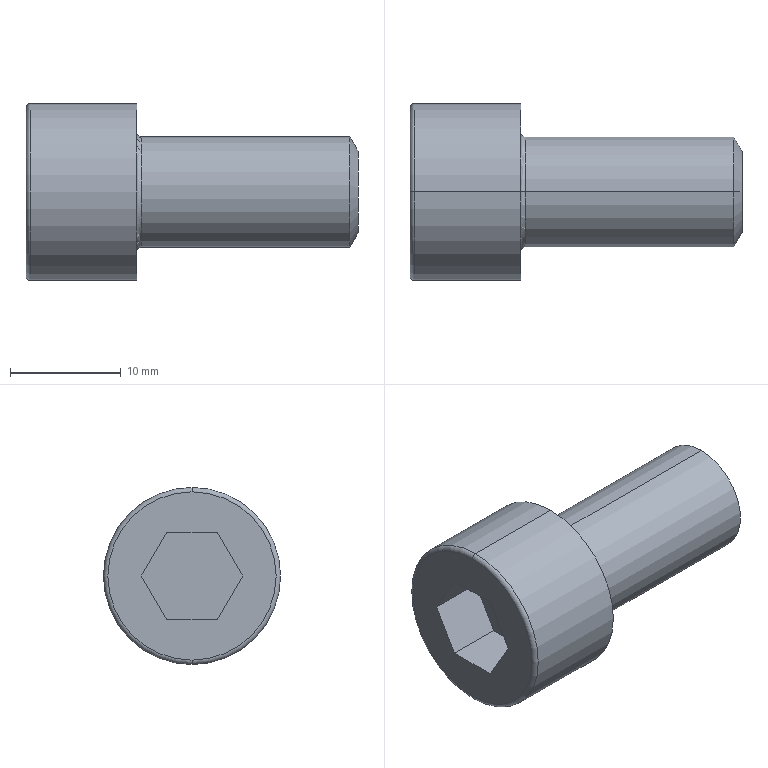Part | SolidWorks | features BlendCut 1, Cut 1, Fillet 1, LPattern 1, RevCut 1, Revolution 1 | 1 solid | 20 faces | box 30 x 16 x 16 mm | volume 3295 mm3 | plane 10 | torus 4 | cylinder 4 | cone 2 | commonest cylinder face diameters 10 x2 16 x2
STEP:
#1=CARTESIAN_POINT('',(30.,0.,3.701));
#2=VERTEX_POINT('',#1);
#3=CARTESIAN_POINT('',(30.,0.,-3.701));
#4=VERTEX_POINT('',#3);
#5=CARTESIAN_POINT('',(30.,0.,0.));
#6=DIRECTION('',(-1.,0.,0.));
#7=DIRECTION('',(0.,0.,1.));
#8=AXIS2_PLACEMENT_3D('',#5,#6,#7);
#9=CIRCLE('',#8,3.701);
#10=EDGE_CURVE('',#2,#4,#9,.T.);
#11=ORIENTED_EDGE('',*,*,#10,.T.);
#12=CARTESIAN_POINT('',(29.25,0.,-5.));
#13=VERTEX_POINT('',#12);
#14=CARTESIAN_POINT('',(29.25,0.,-5.));
#15=DIRECTION('',(-0.5,0.,-0.866));
#16=VECTOR('',#15,1000.);
#17=LINE('',#14,#16);
#18=EDGE_CURVE('',#4,#13,#17,.T.);
#19=ORIENTED_EDGE('',*,*,#18,.T.);
#20=CARTESIAN_POINT('',(29.25,0.,5.));
#21=VERTEX_POINT('',#20);
#22=CARTESIAN_POINT('',(29.25,0.,0.));
#23=DIRECTION('',(-1.,0.,0.));
#24=DIRECTION('',(0.,0.,1.));
#25=AXIS2_PLACEMENT_3D('',#22,#23,#24);
#26=CIRCLE('',#25,5.);
#27=EDGE_CURVE('',#21,#13,#26,.T.);
#28=ORIENTED_EDGE('',*,*,#27,.F.);
#29=CARTESIAN_POINT('',(29.25,0.,5.));
#30=DIRECTION('',(-0.5,0.,0.866));
#31=VECTOR('',#30,1000.);
#32=LINE('',#29,#31);
#33=EDGE_CURVE('',#2,#21,#32,.T.);
#34=ORIENTED_EDGE('',*,*,#33,.F.);
#35=EDGE_LOOP('',(#11,#19,#28,#34));
#36=FACE_OUTER_BOUND('',#35,.T.);
#37=CARTESIAN_POINT('',(29.25,0.,0.));
#38=DIRECTION('',(-1.,0.,0.));
#39=DIRECTION('',(0.,0.,1.));
#40=AXIS2_PLACEMENT_3D('',#37,#38,#39);
#41=CONICAL_SURFACE('',#40,5.,1.047);
#42=ADVANCED_FACE('',(#36),#41,.T.);
#43=CARTESIAN_POINT('',(0.4,0.,-8.));
#44=VERTEX_POINT('',#43);
#45=CARTESIAN_POINT('',(0.4,0.,8.));
#46=VERTEX_POINT('',#45);
#47=CARTESIAN_POINT('',(0.4,0.,0.));
#48=DIRECTION('',(1.,0.,0.));
#49=DIRECTION('',(0.,0.,1.));
#50=AXIS2_PLACEMENT_3D('',#47,#48,#49);
#51=CIRCLE('',#50,8.);
#52=EDGE_CURVE('',#44,#46,#51,.T.);
#53=ORIENTED_EDGE('',*,*,#52,.F.);
#54=CARTESIAN_POINT('',(0.,0.,-7.6));
#55=VERTEX_POINT('',#54);
#56=CARTESIAN_POINT('',(0.4,0.,-7.6));
#57=DIRECTION('',(0.,1.,0.));
#58=DIRECTION('',(0.,0.,1.));
#59=AXIS2_PLACEMENT_3D('',#56,#57,#58);
#60=CIRCLE('',#59,0.4);
#61=EDGE_CURVE('',#44,#55,#60,.T.);
#62=ORIENTED_EDGE('',*,*,#61,.T.);
#63=CARTESIAN_POINT('',(0.,0.,7.6));
#64=VERTEX_POINT('',#63);
#65=CARTESIAN_POINT('',(0.,0.,0.));
#66=DIRECTION('',(-1.,0.,0.));
#67=DIRECTION('',(0.,0.,1.));
#68=AXIS2_PLACEMENT_3D('',#65,#66,#67);
#69=CIRCLE('',#68,7.6);
#70=EDGE_CURVE('',#64,#55,#69,.T.);
#71=ORIENTED_EDGE('',*,*,#70,.F.);
#72=CARTESIAN_POINT('',(0.4,0.,7.6));
#73=DIRECTION('',(0.,-1.,0.));
#74=DIRECTION('',(0.,0.,-1.));
#75=AXIS2_PLACEMENT_3D('',#72,#73,#74);
#76=CIRCLE('',#75,0.4);
#77=EDGE_CURVE('',#46,#64,#76,.T.);
#78=ORIENTED_EDGE('',*,*,#77,.F.);
#79=EDGE_LOOP('',(#53,#62,#71,#78));
#80=FACE_OUTER_BOUND('',#79,.T.);
#81=CARTESIAN_POINT('',(0.4,0.,0.));
#82=DIRECTION('',(-1.,0.,0.));
#83=DIRECTION('',(0.,0.,1.));
#84=AXIS2_PLACEMENT_3D('',#81,#82,#83);
#85=TOROIDAL_SURFACE('',#84,7.6,0.4);
#86=ADVANCED_FACE('',(#80),#85,.T.);
#87=CARTESIAN_POINT('',(10.4,0.,5.));
#88=VERTEX_POINT('',#87);
#89=CARTESIAN_POINT('',(10.4,0.,-5.));
#90=VERTEX_POINT('',#89);
#91=CARTESIAN_POINT('',(10.4,0.,0.));
#92=DIRECTION('',(1.,0.,0.));
#93=DIRECTION('',(0.,0.,-1.));
#94=AXIS2_PLACEMENT_3D('',#91,#92,#93);
#95=CIRCLE('',#94,5.);
#96=EDGE_CURVE('',#88,#90,#95,.T.);
#97=ORIENTED_EDGE('',*,*,#96,.F.);
#98=CARTESIAN_POINT('',(10.,0.,5.4));
#99=VERTEX_POINT('',#98);
#100=CARTESIAN_POINT('',(10.4,0.,5.4));
#101=DIRECTION('',(0.,1.,0.));
#102=DIRECTION('',(0.,0.,1.));
#103=AXIS2_PLACEMENT_3D('',#100,#101,#102);
#104=CIRCLE('',#103,0.4);
#105=EDGE_CURVE('',#88,#99,#104,.T.);
#106=ORIENTED_EDGE('',*,*,#105,.T.);
#107=CARTESIAN_POINT('',(10.,0.,-5.4));
#108=VERTEX_POINT('',#107);
#109=CARTESIAN_POINT('',(10.,0.,0.));
#110=DIRECTION('',(1.,0.,0.));
#111=DIRECTION('',(0.,0.,-1.));
#112=AXIS2_PLACEMENT_3D('',#109,#110,#111);
#113=CIRCLE('',#112,5.4);
#114=EDGE_CURVE('',#99,#108,#113,.T.);
#115=ORIENTED_EDGE('',*,*,#114,.T.);
#116=CARTESIAN_POINT('',(10.4,0.,-5.4));
#117=DIRECTION('',(0.,-1.,0.));
#118=DIRECTION('',(0.,0.,-1.));
#119=AXIS2_PLACEMENT_3D('',#116,#117,#118);
#120=CIRCLE('',#119,0.4);
#121=EDGE_CURVE('',#90,#108,#120,.T.);
#122=ORIENTED_EDGE('',*,*,#121,.F.);
#123=EDGE_LOOP('',(#97,#106,#115,#122));
#124=FACE_OUTER_BOUND('',#123,.T.);
#125=CARTESIAN_POINT('',(10.4,0.,0.));
#126=DIRECTION('',(1.,0.,0.));
#127=DIRECTION('',(0.,0.,-1.));
#128=AXIS2_PLACEMENT_3D('',#125,#126,#127);
#129=TOROIDAL_SURFACE('',#128,5.4,0.4);
#130=ADVANCED_FACE('',(#124),#129,.F.);
#131=ORIENTED_EDGE('',*,*,#52,.T.);
#132=CARTESIAN_POINT('',(10.,0.,8.));
#133=VERTEX_POINT('',#132);
#134=CARTESIAN_POINT('',(0.,0.,8.));
#135=DIRECTION('',(1.,0.,0.));
#136=VECTOR('',#135,1000.);
#137=LINE('',#134,#136);
#138=EDGE_CURVE('',#46,#133,#137,.T.);
#139=ORIENTED_EDGE('',*,*,#138,.T.);
#140=CARTESIAN_POINT('',(10.,0.,-8.));
#141=VERTEX_POINT('',#140);
#142=CARTESIAN_POINT('',(10.,0.,0.));
#143=DIRECTION('',(1.,0.,0.));
#144=DIRECTION('',(0.,0.,-1.));
#145=AXIS2_PLACEMENT_3D('',#142,#143,#144);
#146=CIRCLE('',#145,8.);
#147=EDGE_CURVE('',#141,#133,#146,.T.);
#148=ORIENTED_EDGE('',*,*,#147,.F.);
#149=CARTESIAN_POINT('',(0.,0.,-8.));
#150=DIRECTION('',(1.,0.,0.));
#151=VECTOR('',#150,1000.);
#152=LINE('',#149,#151);
#153=EDGE_CURVE('',#44,#141,#152,.T.);
#154=ORIENTED_EDGE('',*,*,#153,.F.);
#155=EDGE_LOOP('',(#131,#139,#148,#154));
#156=FACE_OUTER_BOUND('',#155,.T.);
#157=CARTESIAN_POINT('',(0.,0.,0.));
#158=DIRECTION('',(1.,0.,0.));
#159=DIRECTION('',(0.,0.,-1.));
#160=AXIS2_PLACEMENT_3D('',#157,#158,#159);
#161=CYLINDRICAL_SURFACE('',#160,8.);
#162=ADVANCED_FACE('',(#156),#161,.T.);
#163=CARTESIAN_POINT('',(10.4,0.,0.));
#164=DIRECTION('',(1.,0.,0.));
#165=DIRECTION('',(0.,0.,-1.));
#166=AXIS2_PLACEMENT_3D('',#163,#164,#165);
#167=CIRCLE('',#166,5.);
#168=EDGE_CURVE('',#90,#88,#167,.T.);
#169=ORIENTED_EDGE('',*,*,#168,.T.);
#170=CARTESIAN_POINT('',(0.,0.,5.));
#171=DIRECTION('',(1.,0.,0.));
#172=VECTOR('',#171,1000.);
#173=LINE('',#170,#172);
#174=EDGE_CURVE('',#88,#21,#173,.T.);
#175=ORIENTED_EDGE('',*,*,#174,.T.);
#176=ORIENTED_EDGE('',*,*,#27,.T.);
#177=CARTESIAN_POINT('',(0.,0.,-5.));
#178=DIRECTION('',(1.,0.,0.));
#179=VECTOR('',#178,1000.);
#180=LINE('',#177,#179);
#181=EDGE_CURVE('',#90,#13,#180,.T.);
#182=ORIENTED_EDGE('',*,*,#181,.F.);
#183=EDGE_LOOP('',(#169,#175,#176,#182));
#184=FACE_OUTER_BOUND('',#183,.T.);
#185=CARTESIAN_POINT('',(0.,0.,0.));
#186=DIRECTION('',(1.,0.,0.));
#187=DIRECTION('',(0.,0.,-1.));
#188=AXIS2_PLACEMENT_3D('',#185,#186,#187);
#189=CYLINDRICAL_SURFACE('',#188,5.);
#190=ADVANCED_FACE('',(#184),#189,.T.);
#191=ORIENTED_EDGE('',*,*,#174,.F.);
#192=ORIENTED_EDGE('',*,*,#96,.T.);
#193=ORIENTED_EDGE('',*,*,#181,.T.);
#194=CARTESIAN_POINT('',(29.25,0.,0.));
#195=DIRECTION('',(-1.,0.,0.));
#196=DIRECTION('',(0.,0.,1.));
#197=AXIS2_PLACEMENT_3D('',#194,#195,#196);
#198=CIRCLE('',#197,5.);
#199=EDGE_CURVE('',#13,#21,#198,.T.);
#200=ORIENTED_EDGE('',*,*,#199,.T.);
#201=EDGE_LOOP('',(#191,#192,#193,#200));
#202=FACE_OUTER_BOUND('',#201,.T.);
#203=CARTESIAN_POINT('',(0.,0.,0.));
#204=DIRECTION('',(1.,0.,0.));
#205=DIRECTION('',(0.,0.,-1.));
#206=AXIS2_PLACEMENT_3D('',#203,#204,#205);
#207=CYLINDRICAL_SURFACE('',#206,5.);
#208=ADVANCED_FACE('',(#202),#207,.T.);
#209=ORIENTED_EDGE('',*,*,#70,.T.);
#210=CARTESIAN_POINT('',(0.,0.,0.));
#211=DIRECTION('',(-1.,0.,0.));
#212=DIRECTION('',(0.,0.,1.));
#213=AXIS2_PLACEMENT_3D('',#210,#211,#212);
#214=CIRCLE('',#213,7.6);
#215=EDGE_CURVE('',#55,#64,#214,.T.);
#216=ORIENTED_EDGE('',*,*,#215,.T.);
#217=EDGE_LOOP('',(#209,#216));
#218=FACE_OUTER_BOUND('',#217,.T.);
#219=CARTESIAN_POINT('',(0.,-4.575,0.));
#220=VERTEX_POINT('',#219);
#221=CARTESIAN_POINT('',(0.,-2.288,3.962));
#222=VERTEX_POINT('',#221);
#223=CARTESIAN_POINT('',(0.,-4.575,0.));
#224=DIRECTION('',(0.,0.5,0.866));
#225=VECTOR('',#224,1000.);
#226=LINE('',#223,#225);
#227=EDGE_CURVE('',#220,#222,#226,.T.);
#228=ORIENTED_EDGE('',*,*,#227,.F.);
#229=CARTESIAN_POINT('',(0.,-2.288,-3.962));
#230=VERTEX_POINT('',#229);
#231=CARTESIAN_POINT('',(0.,-2.288,-3.962));
#232=DIRECTION('',(0.,-0.5,0.866));
#233=VECTOR('',#232,1000.);
#234=LINE('',#231,#233);
#235=EDGE_CURVE('',#230,#220,#234,.T.);
#236=ORIENTED_EDGE('',*,*,#235,.F.);
#237=CARTESIAN_POINT('',(0.,2.288,-3.962));
#238=VERTEX_POINT('',#237);
#239=CARTESIAN_POINT('',(0.,2.288,-3.962));
#240=DIRECTION('',(0.,-1.,0.));
#241=VECTOR('',#240,1000.);
#242=LINE('',#239,#241);
#243=EDGE_CURVE('',#238,#230,#242,.T.);
#244=ORIENTED_EDGE('',*,*,#243,.F.);
#245=CARTESIAN_POINT('',(0.,4.575,0.));
#246=VERTEX_POINT('',#245);
#247=CARTESIAN_POINT('',(0.,4.575,0.));
#248=DIRECTION('',(0.,-0.5,-0.866));
#249=VECTOR('',#248,1000.);
#250=LINE('',#247,#249);
#251=EDGE_CURVE('',#246,#238,#250,.T.);
#252=ORIENTED_EDGE('',*,*,#251,.F.);
#253=CARTESIAN_POINT('',(0.,2.288,3.962));
#254=VERTEX_POINT('',#253);
#255=CARTESIAN_POINT('',(0.,2.288,3.962));
#256=DIRECTION('',(0.,0.5,-0.866));
#257=VECTOR('',#256,1000.);
#258=LINE('',#255,#257);
#259=EDGE_CURVE('',#254,#246,#258,.T.);
#260=ORIENTED_EDGE('',*,*,#259,.F.);
#261=CARTESIAN_POINT('',(0.,-2.288,3.962));
#262=DIRECTION('',(0.,1.,0.));
#263=VECTOR('',#262,1000.);
#264=LINE('',#261,#263);
#265=EDGE_CURVE('',#222,#254,#264,.T.);
#266=ORIENTED_EDGE('',*,*,#265,.F.);
#267=EDGE_LOOP('',(#228,#236,#244,#252,#260,#266));
#268=FACE_BOUND('',#267,.T.);
#269=CARTESIAN_POINT('',(0.,0.,0.));
#270=DIRECTION('',(-1.,0.,0.));
#271=DIRECTION('',(0.,0.,1.));
#272=AXIS2_PLACEMENT_3D('',#269,#270,#271);
#273=PLANE('',#272);
#274=ADVANCED_FACE('',(#218,#268),#273,.T.);
#275=ORIENTED_EDGE('',*,*,#138,.F.);
#276=CARTESIAN_POINT('',(0.4,0.,0.));
#277=DIRECTION('',(1.,0.,0.));
#278=DIRECTION('',(0.,0.,1.));
#279=AXIS2_PLACEMENT_3D('',#276,#277,#278);
#280=CIRCLE('',#279,8.);
#281=EDGE_CURVE('',#46,#44,#280,.T.);
#282=ORIENTED_EDGE('',*,*,#281,.T.);
#283=ORIENTED_EDGE('',*,*,#153,.T.);
#284=CARTESIAN_POINT('',(10.,0.,0.));
#285=DIRECTION('',(1.,0.,0.));
#286=DIRECTION('',(0.,0.,-1.));
#287=AXIS2_PLACEMENT_3D('',#284,#285,#286);
#288=CIRCLE('',#287,8.);
#289=EDGE_CURVE('',#133,#141,#288,.T.);
#290=ORIENTED_EDGE('',*,*,#289,.F.);
#291=EDGE_LOOP('',(#275,#282,#283,#290));
#292=FACE_OUTER_BOUND('',#291,.T.);
#293=CARTESIAN_POINT('',(0.,0.,0.));
#294=DIRECTION('',(1.,0.,0.));
#295=DIRECTION('',(0.,0.,-1.));
#296=AXIS2_PLACEMENT_3D('',#293,#294,#295);
#297=CYLINDRICAL_SURFACE('',#296,8.);
#298=ADVANCED_FACE('',(#292),#297,.T.);
#299=ORIENTED_EDGE('',*,*,#147,.T.);
#300=ORIENTED_EDGE('',*,*,#289,.T.);
#301=EDGE_LOOP('',(#299,#300));
#302=FACE_OUTER_BOUND('',#301,.T.);
#303=CARTESIAN_POINT('',(10.,0.,0.));
#304=DIRECTION('',(1.,0.,0.));
#305=DIRECTION('',(0.,0.,-1.));
#306=AXIS2_PLACEMENT_3D('',#303,#304,#305);
#307=CIRCLE('',#306,5.4);
#308=EDGE_CURVE('',#108,#99,#307,.T.);
#309=ORIENTED_EDGE('',*,*,#308,.F.);
#310=ORIENTED_EDGE('',*,*,#114,.F.);
#311=EDGE_LOOP('',(#309,#310));
#312=FACE_BOUND('',#311,.T.);
#313=CARTESIAN_POINT('',(10.,8.,0.));
#314=DIRECTION('',(1.,0.,0.));
#315=DIRECTION('',(0.,0.,-1.));
#316=AXIS2_PLACEMENT_3D('',#313,#314,#315);
#317=PLANE('',#316);
#318=ADVANCED_FACE('',(#302,#312),#317,.T.);
#319=ORIENTED_EDGE('',*,*,#105,.F.);
#320=ORIENTED_EDGE('',*,*,#168,.F.);
#321=ORIENTED_EDGE('',*,*,#121,.T.);
#322=ORIENTED_EDGE('',*,*,#308,.T.);
#323=EDGE_LOOP('',(#319,#320,#321,#322));
#324=FACE_OUTER_BOUND('',#323,.T.);
#325=CARTESIAN_POINT('',(10.4,0.,0.));
#326=DIRECTION('',(1.,0.,0.));
#327=DIRECTION('',(0.,0.,-1.));
#328=AXIS2_PLACEMENT_3D('',#325,#326,#327);
#329=TOROIDAL_SURFACE('',#328,5.4,0.4);
#330=ADVANCED_FACE('',(#324),#329,.F.);
#331=ORIENTED_EDGE('',*,*,#227,.T.);
#332=CARTESIAN_POINT('',(5.,-2.288,3.962));
#333=VERTEX_POINT('',#332);
#334=CARTESIAN_POINT('',(5.,-2.288,3.962));
#335=DIRECTION('',(-1.,0.,0.));
#336=VECTOR('',#335,1000.);
#337=LINE('',#334,#336);
#338=EDGE_CURVE('',#333,#222,#337,.T.);
#339=ORIENTED_EDGE('',*,*,#338,.F.);
#340=CARTESIAN_POINT('',(5.,-4.575,0.));
#341=VERTEX_POINT('',#340);
#342=CARTESIAN_POINT('',(5.,-4.575,0.));
#343=DIRECTION('',(0.,0.5,0.866));
#344=VECTOR('',#343,1000.);
#345=LINE('',#342,#344);
#346=EDGE_CURVE('',#341,#333,#345,.T.);
#347=ORIENTED_EDGE('',*,*,#346,.F.);
#348=CARTESIAN_POINT('',(5.,-4.575,0.));
#349=DIRECTION('',(-1.,0.,0.));
#350=VECTOR('',#349,1000.);
#351=LINE('',#348,#350);
#352=EDGE_CURVE('',#341,#220,#351,.T.);
#353=ORIENTED_EDGE('',*,*,#352,.T.);
#354=EDGE_LOOP('',(#331,#339,#347,#353));
#355=FACE_OUTER_BOUND('',#354,.T.);
#356=CARTESIAN_POINT('',(5.,-4.575,0.));
#357=DIRECTION('',(0.,-0.866,0.5));
#358=DIRECTION('',(0.,-0.5,-0.866));
#359=AXIS2_PLACEMENT_3D('',#356,#357,#358);
#360=PLANE('',#359);
#361=ADVANCED_FACE('',(#355),#360,.F.);
#362=ORIENTED_EDGE('',*,*,#235,.T.);
#363=ORIENTED_EDGE('',*,*,#352,.F.);
#364=CARTESIAN_POINT('',(5.,-2.288,-3.962));
#365=VERTEX_POINT('',#364);
#366=CARTESIAN_POINT('',(5.,-2.288,-3.962));
#367=DIRECTION('',(0.,-0.5,0.866));
#368=VECTOR('',#367,1000.);
#369=LINE('',#366,#368);
#370=EDGE_CURVE('',#365,#341,#369,.T.);
#371=ORIENTED_EDGE('',*,*,#370,.F.);
#372=CARTESIAN_POINT('',(5.,-2.288,-3.962));
#373=DIRECTION('',(-1.,0.,0.));
#374=VECTOR('',#373,1000.);
#375=LINE('',#372,#374);
#376=EDGE_CURVE('',#365,#230,#375,.T.);
#377=ORIENTED_EDGE('',*,*,#376,.T.);
#378=EDGE_LOOP('',(#362,#363,#371,#377));
#379=FACE_OUTER_BOUND('',#378,.T.);
#380=CARTESIAN_POINT('',(5.,-2.288,-3.962));
#381=DIRECTION('',(0.,-0.866,-0.5));
#382=DIRECTION('',(0.,0.5,-0.866));
#383=AXIS2_PLACEMENT_3D('',#380,#381,#382);
#384=PLANE('',#383);
#385=ADVANCED_FACE('',(#379),#384,.F.);
#386=ORIENTED_EDGE('',*,*,#243,.T.);
#387=ORIENTED_EDGE('',*,*,#376,.F.);
#388=CARTESIAN_POINT('',(5.,2.288,-3.962));
#389=VERTEX_POINT('',#388);
#390=CARTESIAN_POINT('',(5.,2.288,-3.962));
#391=DIRECTION('',(0.,-1.,0.));
#392=VECTOR('',#391,1000.);
#393=LINE('',#390,#392);
#394=EDGE_CURVE('',#389,#365,#393,.T.);
#395=ORIENTED_EDGE('',*,*,#394,.F.);
#396=CARTESIAN_POINT('',(5.,2.288,-3.962));
#397=DIRECTION('',(-1.,0.,0.));
#398=VECTOR('',#397,1000.);
#399=LINE('',#396,#398);
#400=EDGE_CURVE('',#389,#238,#399,.T.);
#401=ORIENTED_EDGE('',*,*,#400,.T.);
#402=EDGE_LOOP('',(#386,#387,#395,#401));
#403=FACE_OUTER_BOUND('',#402,.T.);
#404=CARTESIAN_POINT('',(5.,2.288,-3.962));
#405=DIRECTION('',(0.,0.,-1.));
#406=DIRECTION('',(0.,1.,0.));
#407=AXIS2_PLACEMENT_3D('',#404,#405,#406);
#408=PLANE('',#407);
#409=ADVANCED_FACE('',(#403),#408,.F.);
#410=ORIENTED_EDGE('',*,*,#251,.T.);
#411=ORIENTED_EDGE('',*,*,#400,.F.);
#412=CARTESIAN_POINT('',(5.,4.575,0.));
#413=VERTEX_POINT('',#412);
#414=CARTESIAN_POINT('',(5.,4.575,0.));
#415=DIRECTION('',(0.,-0.5,-0.866));
#416=VECTOR('',#415,1000.);
#417=LINE('',#414,#416);
#418=EDGE_CURVE('',#413,#389,#417,.T.);
#419=ORIENTED_EDGE('',*,*,#418,.F.);
#420=CARTESIAN_POINT('',(5.,4.575,0.));
#421=DIRECTION('',(-1.,0.,0.));
#422=VECTOR('',#421,1000.);
#423=LINE('',#420,#422);
#424=EDGE_CURVE('',#413,#246,#423,.T.);
#425=ORIENTED_EDGE('',*,*,#424,.T.);
#426=EDGE_LOOP('',(#410,#411,#419,#425));
#427=FACE_OUTER_BOUND('',#426,.T.);
#428=CARTESIAN_POINT('',(5.,4.575,0.));
#429=DIRECTION('',(0.,0.866,-0.5));
#430=DIRECTION('',(0.,0.5,0.866));
#431=AXIS2_PLACEMENT_3D('',#428,#429,#430);
#432=PLANE('',#431);
#433=ADVANCED_FACE('',(#427),#432,.F.);
#434=ORIENTED_EDGE('',*,*,#259,.T.);
#435=ORIENTED_EDGE('',*,*,#424,.F.);
#436=CARTESIAN_POINT('',(5.,2.288,3.962));
#437=VERTEX_POINT('',#436);
#438=CARTESIAN_POINT('',(5.,2.288,3.962));
#439=DIRECTION('',(0.,0.5,-0.866));
#440=VECTOR('',#439,1000.);
#441=LINE('',#438,#440);
#442=EDGE_CURVE('',#437,#413,#441,.T.);
#443=ORIENTED_EDGE('',*,*,#442,.F.);
#444=CARTESIAN_POINT('',(5.,2.288,3.962));
#445=DIRECTION('',(-1.,0.,0.));
#446=VECTOR('',#445,1000.);
#447=LINE('',#444,#446);
#448=EDGE_CURVE('',#437,#254,#447,.T.);
#449=ORIENTED_EDGE('',*,*,#448,.T.);
#450=EDGE_LOOP('',(#434,#435,#443,#449));
#451=FACE_OUTER_BOUND('',#450,.T.);
#452=CARTESIAN_POINT('',(5.,2.288,3.962));
#453=DIRECTION('',(0.,0.866,0.5));
#454=DIRECTION('',(0.,-0.5,0.866));
#455=AXIS2_PLACEMENT_3D('',#452,#453,#454);
#456=PLANE('',#455);
#457=ADVANCED_FACE('',(#451),#456,.F.);
#458=ORIENTED_EDGE('',*,*,#265,.T.);
#459=ORIENTED_EDGE('',*,*,#448,.F.);
#460=CARTESIAN_POINT('',(5.,-2.288,3.962));
#461=DIRECTION('',(0.,1.,0.));
#462=VECTOR('',#461,1000.);
#463=LINE('',#460,#462);
#464=EDGE_CURVE('',#333,#437,#463,.T.);
#465=ORIENTED_EDGE('',*,*,#464,.F.);
#466=ORIENTED_EDGE('',*,*,#338,.T.);
#467=EDGE_LOOP('',(#458,#459,#465,#466));
#468=FACE_OUTER_BOUND('',#467,.T.);
#469=CARTESIAN_POINT('',(5.,-2.288,3.962));
#470=DIRECTION('',(0.,0.,1.));
#471=DIRECTION('',(0.,-1.,0.));
#472=AXIS2_PLACEMENT_3D('',#469,#470,#471);
#473=PLANE('',#472);
#474=ADVANCED_FACE('',(#468),#473,.F.);
#475=ORIENTED_EDGE('',*,*,#346,.T.);
#476=ORIENTED_EDGE('',*,*,#464,.T.);
#477=ORIENTED_EDGE('',*,*,#442,.T.);
#478=ORIENTED_EDGE('',*,*,#418,.T.);
#479=ORIENTED_EDGE('',*,*,#394,.T.);
#480=ORIENTED_EDGE('',*,*,#370,.T.);
#481=EDGE_LOOP('',(#475,#476,#477,#478,#479,#480));
#482=FACE_OUTER_BOUND('',#481,.T.);
#483=CARTESIAN_POINT('',(5.,-2.288,3.962));
#484=DIRECTION('',(-1.,0.,0.));
#485=DIRECTION('',(0.,0.,1.));
#486=AXIS2_PLACEMENT_3D('',#483,#484,#485);
#487=PLANE('',#486);
#488=ADVANCED_FACE('',(#482),#487,.T.);
#489=ORIENTED_EDGE('',*,*,#61,.F.);
#490=ORIENTED_EDGE('',*,*,#281,.F.);
#491=ORIENTED_EDGE('',*,*,#77,.T.);
#492=ORIENTED_EDGE('',*,*,#215,.F.);
#493=EDGE_LOOP('',(#489,#490,#491,#492));
#494=FACE_OUTER_BOUND('',#493,.T.);
#495=CARTESIAN_POINT('',(0.4,0.,0.));
#496=DIRECTION('',(-1.,0.,0.));
#497=DIRECTION('',(0.,0.,1.));
#498=AXIS2_PLACEMENT_3D('',#495,#496,#497);
#499=TOROIDAL_SURFACE('',#498,7.6,0.4);
#500=ADVANCED_FACE('',(#494),#499,.T.);
#501=ORIENTED_EDGE('',*,*,#18,.F.);
#502=CARTESIAN_POINT('',(30.,0.,0.));
#503=DIRECTION('',(-1.,0.,0.));
#504=DIRECTION('',(0.,0.,1.));
#505=AXIS2_PLACEMENT_3D('',#502,#503,#504);
#506=CIRCLE('',#505,3.701);
#507=EDGE_CURVE('',#4,#2,#506,.T.);
#508=ORIENTED_EDGE('',*,*,#507,.T.);
#509=ORIENTED_EDGE('',*,*,#33,.T.);
#510=ORIENTED_EDGE('',*,*,#199,.F.);
#511=EDGE_LOOP('',(#501,#508,#509,#510));
#512=FACE_OUTER_BOUND('',#511,.T.);
#513=CARTESIAN_POINT('',(29.25,0.,0.));
#514=DIRECTION('',(-1.,0.,0.));
#515=DIRECTION('',(0.,0.,1.));
#516=AXIS2_PLACEMENT_3D('',#513,#514,#515);
#517=CONICAL_SURFACE('',#516,5.,1.047);
#518=ADVANCED_FACE('',(#512),#517,.T.);
#519=ORIENTED_EDGE('',*,*,#10,.F.);
#520=ORIENTED_EDGE('',*,*,#507,.F.);
#521=EDGE_LOOP('',(#519,#520));
#522=FACE_OUTER_BOUND('',#521,.T.);
#523=CARTESIAN_POINT('',(30.,5.,0.));
#524=DIRECTION('',(1.,0.,0.));
#525=DIRECTION('',(0.,0.,-1.));
#526=AXIS2_PLACEMENT_3D('',#523,#524,#525);
#527=PLANE('',#526);
#528=ADVANCED_FACE('',(#522),#527,.T.);
#529=CLOSED_SHELL('',(#42,#86,#130,#162,#190,#208,#274,#298,#318,#330,#361,#385,#409,#433,#457,#474,#488,#500,#518,#528));
#530=MANIFOLD_SOLID_BREP('',#529);
#531=CARTESIAN_POINT('',(0.,0.,0.));
#532=DIRECTION('',(0.,0.,1.));
#533=DIRECTION('',(1.,0.,0.));
#534=AXIS2_PLACEMENT_3D('',#531,#532,#533);
#535=(LENGTH_UNIT()NAMED_UNIT(*)SI_UNIT(.MILLI.,.METRE.));
#536=UNCERTAINTY_MEASURE_WITH_UNIT(LENGTH_MEASURE(0.00001),#535,'','');
#537=(NAMED_UNIT(*)PLANE_ANGLE_UNIT()SI_UNIT($,.RADIAN.));
#538=(NAMED_UNIT(*)SI_UNIT($,.STERADIAN.)SOLID_ANGLE_UNIT());
#539=(GEOMETRIC_REPRESENTATION_CONTEXT(3)GLOBAL_UNCERTAINTY_ASSIGNED_CONTEXT((#536))GLOBAL_UNIT_ASSIGNED_CONTEXT((#535,#537,#538))REPRESENTATION_CONTEXT('',''));
#540=ADVANCED_BREP_SHAPE_REPRESENTATION('',(#530,#534),#539);